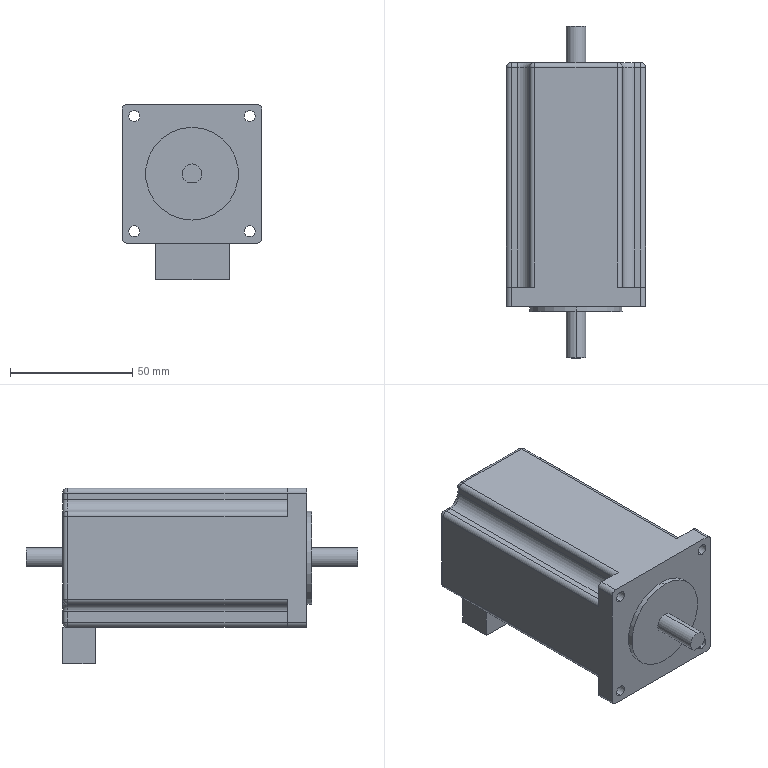Part | NX | features BREP 1 | 1 solid | 82 faces | box 57 x 136 x 72 mm | volume 301973 mm3 | cylinder 41 | plane 29 | sphere 8 | torus 4 | commonest cylinder face diameters 4 x24 4.5 x8 8 x3 10 x3 38 x2 6 x1